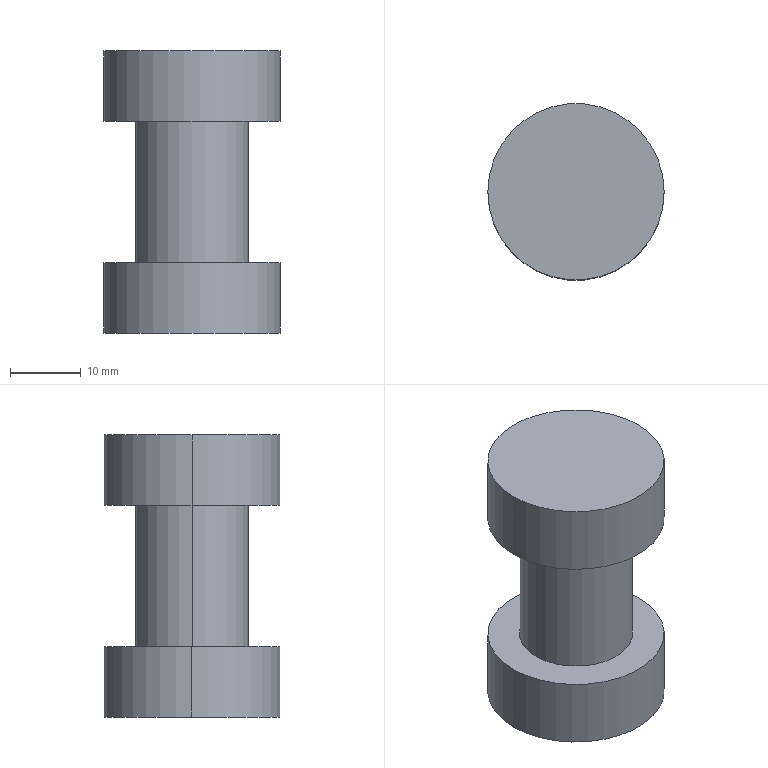Part | SolidWorks | features ICE 2, Extrusion 1 | 1 solid | 10 faces | box 25 x 25 x 40 mm | volume 13839 mm3 | cylinder 6 | plane 4 | commonest cylinder face diameters 25 x4 16 x2
STEP:
#1=CARTESIAN_POINT('',(-12.5,0.,-10.));
#2=VERTEX_POINT('',#1);
#3=CARTESIAN_POINT('',(12.5,0.,-10.));
#4=VERTEX_POINT('',#3);
#5=CARTESIAN_POINT('',(0.,0.,-10.));
#6=DIRECTION('',(0.,0.,-1.));
#7=DIRECTION('',(-1.,0.,0.));
#8=AXIS2_PLACEMENT_3D('',#5,#6,#7);
#9=CIRCLE('',#8,12.5);
#10=EDGE_CURVE('',#2,#4,#9,.T.);
#11=ORIENTED_EDGE('',*,*,#10,.F.);
#12=CARTESIAN_POINT('',(-12.5,0.,0.));
#13=VERTEX_POINT('',#12);
#14=CARTESIAN_POINT('',(-12.5,0.,-10.));
#15=DIRECTION('',(0.,0.,1.));
#16=VECTOR('',#15,1000.);
#17=LINE('',#14,#16);
#18=EDGE_CURVE('',#2,#13,#17,.T.);
#19=ORIENTED_EDGE('',*,*,#18,.T.);
#20=CARTESIAN_POINT('',(12.5,0.,0.));
#21=VERTEX_POINT('',#20);
#22=CARTESIAN_POINT('',(0.,0.,0.));
#23=DIRECTION('',(0.,0.,-1.));
#24=DIRECTION('',(-1.,0.,0.));
#25=AXIS2_PLACEMENT_3D('',#22,#23,#24);
#26=CIRCLE('',#25,12.5);
#27=EDGE_CURVE('',#13,#21,#26,.T.);
#28=ORIENTED_EDGE('',*,*,#27,.T.);
#29=CARTESIAN_POINT('',(12.5,0.,-10.));
#30=DIRECTION('',(0.,0.,1.));
#31=VECTOR('',#30,1000.);
#32=LINE('',#29,#31);
#33=EDGE_CURVE('',#4,#21,#32,.T.);
#34=ORIENTED_EDGE('',*,*,#33,.F.);
#35=EDGE_LOOP('',(#11,#19,#28,#34));
#36=FACE_OUTER_BOUND('',#35,.T.);
#37=CARTESIAN_POINT('',(0.,0.,-10.));
#38=DIRECTION('',(0.,0.,1.));
#39=DIRECTION('',(1.,0.,0.));
#40=AXIS2_PLACEMENT_3D('',#37,#38,#39);
#41=CYLINDRICAL_SURFACE('',#40,12.5);
#42=ADVANCED_FACE('',(#36),#41,.T.);
#43=CARTESIAN_POINT('',(12.5,0.,30.));
#44=VERTEX_POINT('',#43);
#45=CARTESIAN_POINT('',(-12.5,0.,30.));
#46=VERTEX_POINT('',#45);
#47=CARTESIAN_POINT('',(0.,0.,30.));
#48=DIRECTION('',(0.,0.,1.));
#49=DIRECTION('',(1.,0.,0.));
#50=AXIS2_PLACEMENT_3D('',#47,#48,#49);
#51=CIRCLE('',#50,12.5);
#52=EDGE_CURVE('',#44,#46,#51,.T.);
#53=ORIENTED_EDGE('',*,*,#52,.F.);
#54=CARTESIAN_POINT('',(12.5,0.,20.));
#55=VERTEX_POINT('',#54);
#56=CARTESIAN_POINT('',(12.5,0.,30.));
#57=DIRECTION('',(0.,0.,-1.));
#58=VECTOR('',#57,1000.);
#59=LINE('',#56,#58);
#60=EDGE_CURVE('',#44,#55,#59,.T.);
#61=ORIENTED_EDGE('',*,*,#60,.T.);
#62=CARTESIAN_POINT('',(-12.5,0.,20.));
#63=VERTEX_POINT('',#62);
#64=CARTESIAN_POINT('',(0.,0.,20.));
#65=DIRECTION('',(0.,0.,1.));
#66=DIRECTION('',(1.,0.,0.));
#67=AXIS2_PLACEMENT_3D('',#64,#65,#66);
#68=CIRCLE('',#67,12.5);
#69=EDGE_CURVE('',#55,#63,#68,.T.);
#70=ORIENTED_EDGE('',*,*,#69,.T.);
#71=CARTESIAN_POINT('',(-12.5,0.,30.));
#72=DIRECTION('',(0.,0.,-1.));
#73=VECTOR('',#72,1000.);
#74=LINE('',#71,#73);
#75=EDGE_CURVE('',#46,#63,#74,.T.);
#76=ORIENTED_EDGE('',*,*,#75,.F.);
#77=EDGE_LOOP('',(#53,#61,#70,#76));
#78=FACE_OUTER_BOUND('',#77,.T.);
#79=CARTESIAN_POINT('',(0.,0.,30.));
#80=DIRECTION('',(0.,0.,-1.));
#81=DIRECTION('',(-1.,0.,0.));
#82=AXIS2_PLACEMENT_3D('',#79,#80,#81);
#83=CYLINDRICAL_SURFACE('',#82,12.5);
#84=ADVANCED_FACE('',(#78),#83,.T.);
#85=CARTESIAN_POINT('',(8.,0.,20.));
#86=VERTEX_POINT('',#85);
#87=CARTESIAN_POINT('',(-8.,0.,20.));
#88=VERTEX_POINT('',#87);
#89=CARTESIAN_POINT('',(0.,0.,20.));
#90=DIRECTION('',(0.,0.,1.));
#91=DIRECTION('',(1.,0.,0.));
#92=AXIS2_PLACEMENT_3D('',#89,#90,#91);
#93=CIRCLE('',#92,8.);
#94=EDGE_CURVE('',#86,#88,#93,.T.);
#95=ORIENTED_EDGE('',*,*,#94,.F.);
#96=CARTESIAN_POINT('',(8.,0.,0.));
#97=VERTEX_POINT('',#96);
#98=CARTESIAN_POINT('',(8.,0.,20.));
#99=DIRECTION('',(0.,0.,-1.));
#100=VECTOR('',#99,1000.);
#101=LINE('',#98,#100);
#102=EDGE_CURVE('',#86,#97,#101,.T.);
#103=ORIENTED_EDGE('',*,*,#102,.T.);
#104=CARTESIAN_POINT('',(-8.,0.,0.));
#105=VERTEX_POINT('',#104);
#106=CARTESIAN_POINT('',(0.,0.,0.));
#107=DIRECTION('',(0.,0.,1.));
#108=DIRECTION('',(1.,0.,0.));
#109=AXIS2_PLACEMENT_3D('',#106,#107,#108);
#110=CIRCLE('',#109,8.);
#111=EDGE_CURVE('',#97,#105,#110,.T.);
#112=ORIENTED_EDGE('',*,*,#111,.T.);
#113=CARTESIAN_POINT('',(-8.,0.,20.));
#114=DIRECTION('',(0.,0.,-1.));
#115=VECTOR('',#114,1000.);
#116=LINE('',#113,#115);
#117=EDGE_CURVE('',#88,#105,#116,.T.);
#118=ORIENTED_EDGE('',*,*,#117,.F.);
#119=EDGE_LOOP('',(#95,#103,#112,#118));
#120=FACE_OUTER_BOUND('',#119,.T.);
#121=CARTESIAN_POINT('',(0.,0.,20.));
#122=DIRECTION('',(0.,0.,-1.));
#123=DIRECTION('',(-1.,0.,0.));
#124=AXIS2_PLACEMENT_3D('',#121,#122,#123);
#125=CYLINDRICAL_SURFACE('',#124,8.);
#126=ADVANCED_FACE('',(#120),#125,.T.);
#127=ORIENTED_EDGE('',*,*,#102,.F.);
#128=CARTESIAN_POINT('',(0.,0.,20.));
#129=DIRECTION('',(0.,0.,1.));
#130=DIRECTION('',(1.,0.,0.));
#131=AXIS2_PLACEMENT_3D('',#128,#129,#130);
#132=CIRCLE('',#131,8.);
#133=EDGE_CURVE('',#88,#86,#132,.T.);
#134=ORIENTED_EDGE('',*,*,#133,.F.);
#135=ORIENTED_EDGE('',*,*,#117,.T.);
#136=CARTESIAN_POINT('',(0.,0.,0.));
#137=DIRECTION('',(0.,0.,1.));
#138=DIRECTION('',(1.,0.,0.));
#139=AXIS2_PLACEMENT_3D('',#136,#137,#138);
#140=CIRCLE('',#139,8.);
#141=EDGE_CURVE('',#105,#97,#140,.T.);
#142=ORIENTED_EDGE('',*,*,#141,.T.);
#143=EDGE_LOOP('',(#127,#134,#135,#142));
#144=FACE_OUTER_BOUND('',#143,.T.);
#145=CARTESIAN_POINT('',(0.,0.,20.));
#146=DIRECTION('',(0.,0.,-1.));
#147=DIRECTION('',(-1.,0.,0.));
#148=AXIS2_PLACEMENT_3D('',#145,#146,#147);
#149=CYLINDRICAL_SURFACE('',#148,8.);
#150=ADVANCED_FACE('',(#144),#149,.T.);
#151=ORIENTED_EDGE('',*,*,#60,.F.);
#152=CARTESIAN_POINT('',(0.,0.,30.));
#153=DIRECTION('',(0.,0.,1.));
#154=DIRECTION('',(1.,0.,0.));
#155=AXIS2_PLACEMENT_3D('',#152,#153,#154);
#156=CIRCLE('',#155,12.5);
#157=EDGE_CURVE('',#46,#44,#156,.T.);
#158=ORIENTED_EDGE('',*,*,#157,.F.);
#159=ORIENTED_EDGE('',*,*,#75,.T.);
#160=CARTESIAN_POINT('',(0.,0.,20.));
#161=DIRECTION('',(0.,0.,1.));
#162=DIRECTION('',(1.,0.,0.));
#163=AXIS2_PLACEMENT_3D('',#160,#161,#162);
#164=CIRCLE('',#163,12.5);
#165=EDGE_CURVE('',#63,#55,#164,.T.);
#166=ORIENTED_EDGE('',*,*,#165,.T.);
#167=EDGE_LOOP('',(#151,#158,#159,#166));
#168=FACE_OUTER_BOUND('',#167,.T.);
#169=CARTESIAN_POINT('',(0.,0.,30.));
#170=DIRECTION('',(0.,0.,-1.));
#171=DIRECTION('',(-1.,0.,0.));
#172=AXIS2_PLACEMENT_3D('',#169,#170,#171);
#173=CYLINDRICAL_SURFACE('',#172,12.5);
#174=ADVANCED_FACE('',(#168),#173,.T.);
#175=ORIENTED_EDGE('',*,*,#157,.T.);
#176=ORIENTED_EDGE('',*,*,#52,.T.);
#177=EDGE_LOOP('',(#175,#176));
#178=FACE_OUTER_BOUND('',#177,.T.);
#179=CARTESIAN_POINT('',(0.,0.,30.));
#180=DIRECTION('',(0.,0.,1.));
#181=DIRECTION('',(1.,0.,0.));
#182=AXIS2_PLACEMENT_3D('',#179,#180,#181);
#183=PLANE('',#182);
#184=ADVANCED_FACE('',(#178),#183,.T.);
#185=ORIENTED_EDGE('',*,*,#133,.T.);
#186=ORIENTED_EDGE('',*,*,#94,.T.);
#187=EDGE_LOOP('',(#185,#186));
#188=FACE_BOUND('',#187,.T.);
#189=ORIENTED_EDGE('',*,*,#165,.F.);
#190=ORIENTED_EDGE('',*,*,#69,.F.);
#191=EDGE_LOOP('',(#189,#190));
#192=FACE_OUTER_BOUND('',#191,.T.);
#193=CARTESIAN_POINT('',(0.,0.,20.));
#194=DIRECTION('',(0.,0.,1.));
#195=DIRECTION('',(1.,0.,0.));
#196=AXIS2_PLACEMENT_3D('',#193,#194,#195);
#197=PLANE('',#196);
#198=ADVANCED_FACE('',(#188,#192),#197,.F.);
#199=ORIENTED_EDGE('',*,*,#18,.F.);
#200=CARTESIAN_POINT('',(0.,0.,-10.));
#201=DIRECTION('',(0.,0.,-1.));
#202=DIRECTION('',(-1.,0.,0.));
#203=AXIS2_PLACEMENT_3D('',#200,#201,#202);
#204=CIRCLE('',#203,12.5);
#205=EDGE_CURVE('',#4,#2,#204,.T.);
#206=ORIENTED_EDGE('',*,*,#205,.F.);
#207=ORIENTED_EDGE('',*,*,#33,.T.);
#208=CARTESIAN_POINT('',(0.,0.,0.));
#209=DIRECTION('',(0.,0.,-1.));
#210=DIRECTION('',(-1.,0.,0.));
#211=AXIS2_PLACEMENT_3D('',#208,#209,#210);
#212=CIRCLE('',#211,12.5);
#213=EDGE_CURVE('',#21,#13,#212,.T.);
#214=ORIENTED_EDGE('',*,*,#213,.T.);
#215=EDGE_LOOP('',(#199,#206,#207,#214));
#216=FACE_OUTER_BOUND('',#215,.T.);
#217=CARTESIAN_POINT('',(0.,0.,-10.));
#218=DIRECTION('',(0.,0.,1.));
#219=DIRECTION('',(1.,0.,0.));
#220=AXIS2_PLACEMENT_3D('',#217,#218,#219);
#221=CYLINDRICAL_SURFACE('',#220,12.5);
#222=ADVANCED_FACE('',(#216),#221,.T.);
#223=ORIENTED_EDGE('',*,*,#205,.T.);
#224=ORIENTED_EDGE('',*,*,#10,.T.);
#225=EDGE_LOOP('',(#223,#224));
#226=FACE_OUTER_BOUND('',#225,.T.);
#227=CARTESIAN_POINT('',(0.,0.,-10.));
#228=DIRECTION('',(0.,0.,-1.));
#229=DIRECTION('',(-1.,0.,0.));
#230=AXIS2_PLACEMENT_3D('',#227,#228,#229);
#231=PLANE('',#230);
#232=ADVANCED_FACE('',(#226),#231,.T.);
#233=ORIENTED_EDGE('',*,*,#141,.F.);
#234=ORIENTED_EDGE('',*,*,#111,.F.);
#235=EDGE_LOOP('',(#233,#234));
#236=FACE_BOUND('',#235,.T.);
#237=ORIENTED_EDGE('',*,*,#213,.F.);
#238=ORIENTED_EDGE('',*,*,#27,.F.);
#239=EDGE_LOOP('',(#237,#238));
#240=FACE_OUTER_BOUND('',#239,.T.);
#241=CARTESIAN_POINT('',(0.,0.,0.));
#242=DIRECTION('',(0.,0.,-1.));
#243=DIRECTION('',(-1.,0.,0.));
#244=AXIS2_PLACEMENT_3D('',#241,#242,#243);
#245=PLANE('',#244);
#246=ADVANCED_FACE('',(#236,#240),#245,.F.);
#247=CLOSED_SHELL('',(#42,#84,#126,#150,#174,#184,#198,#222,#232,#246));
#248=MANIFOLD_SOLID_BREP('',#247);
#249=CARTESIAN_POINT('',(0.,0.,0.));
#250=DIRECTION('',(0.,0.,1.));
#251=DIRECTION('',(1.,0.,0.));
#252=AXIS2_PLACEMENT_3D('',#249,#250,#251);
#253=(LENGTH_UNIT()NAMED_UNIT(*)SI_UNIT(.MILLI.,.METRE.));
#254=UNCERTAINTY_MEASURE_WITH_UNIT(LENGTH_MEASURE(0.00001),#253,'','');
#255=(NAMED_UNIT(*)PLANE_ANGLE_UNIT()SI_UNIT($,.RADIAN.));
#256=(NAMED_UNIT(*)SI_UNIT($,.STERADIAN.)SOLID_ANGLE_UNIT());
#257=(GEOMETRIC_REPRESENTATION_CONTEXT(3)GLOBAL_UNCERTAINTY_ASSIGNED_CONTEXT((#254))GLOBAL_UNIT_ASSIGNED_CONTEXT((#253,#255,#256))REPRESENTATION_CONTEXT('',''));
#258=ADVANCED_BREP_SHAPE_REPRESENTATION('',(#248,#252),#257);